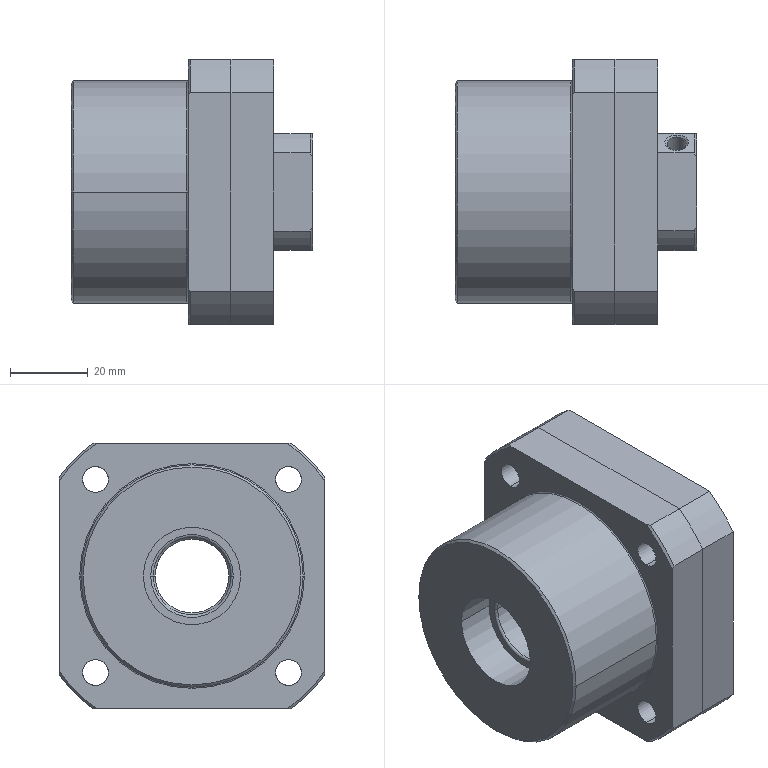Part | NX | 5 solids | 222 faces | box 62 x 68 x 68 mm | volume 148461 mm3 | cylinder 90 | plane 70 | cone 36 | torus 26 | commonest cylinder face diameters 6.6 x16 11 x8 12.9 x8 14 x8 47 x8 85 x8